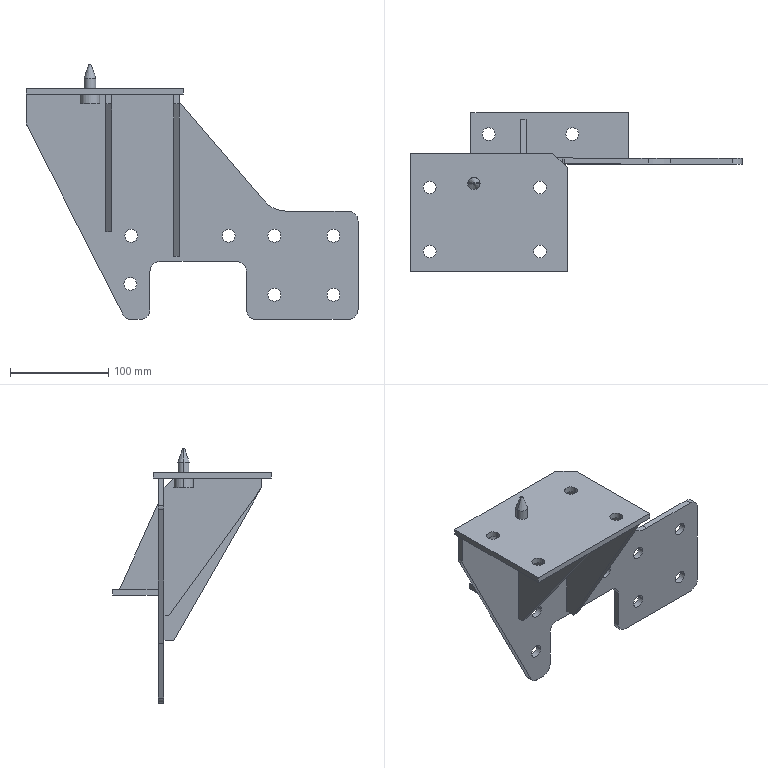Part | NX | features BREP 7 | 7 solids | 97 faces | box 337.5 x 161 x 259 mm | volume 536399 mm3 | plane 52 | cylinder 42 | cone 3 | commonest cylinder face diameters 13 x26 20 x11 12 x2 12.5 x2 60 x1